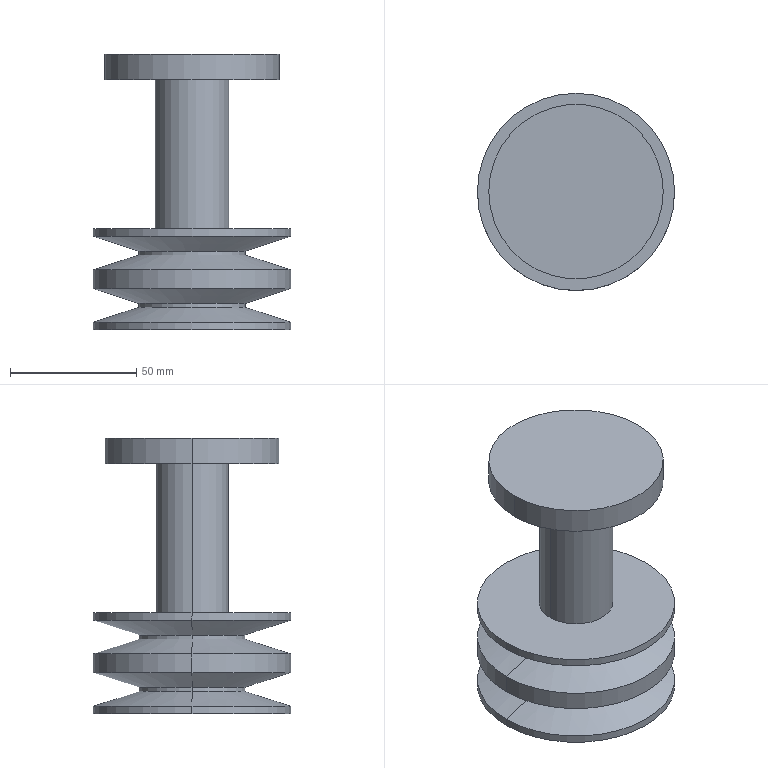Part | SolidWorks | features ICE 6, BaseBody 1 | 1 solid | 38 faces | box 78 x 78 x 109 mm | volume 212709 mm3 | cylinder 18 | cone 11 | plane 9 | commonest cylinder face diameters 78 x6 42 x4 28 x3 29 x2 69 x2 6 x1
STEP:
#1=CARTESIAN_POINT('',(-34.5,0.,109.));
#2=VERTEX_POINT('',#1);
#3=CARTESIAN_POINT('',(34.5,0.,109.));
#4=VERTEX_POINT('',#3);
#5=CARTESIAN_POINT('',(0.,0.,109.));
#6=DIRECTION('',(0.,0.,-1.));
#7=DIRECTION('',(1.,0.,0.));
#8=AXIS2_PLACEMENT_3D('',#5,#6,#7);
#9=CIRCLE('',#8,34.5);
#10=EDGE_CURVE('',#2,#4,#9,.T.);
#11=ORIENTED_EDGE('',*,*,#10,.T.);
#12=CARTESIAN_POINT('',(34.5,0.,99.));
#13=VERTEX_POINT('',#12);
#14=CARTESIAN_POINT('',(34.5,0.,109.));
#15=DIRECTION('',(0.,0.,-1.));
#16=VECTOR('',#15,1000.);
#17=LINE('',#14,#16);
#18=EDGE_CURVE('',#4,#13,#17,.T.);
#19=ORIENTED_EDGE('',*,*,#18,.T.);
#20=CARTESIAN_POINT('',(-34.5,0.,99.));
#21=VERTEX_POINT('',#20);
#22=CARTESIAN_POINT('',(0.,0.,99.));
#23=DIRECTION('',(0.,0.,-1.));
#24=DIRECTION('',(1.,0.,0.));
#25=AXIS2_PLACEMENT_3D('',#22,#23,#24);
#26=CIRCLE('',#25,34.5);
#27=EDGE_CURVE('',#21,#13,#26,.T.);
#28=ORIENTED_EDGE('',*,*,#27,.F.);
#29=CARTESIAN_POINT('',(-34.5,0.,109.));
#30=DIRECTION('',(0.,0.,-1.));
#31=VECTOR('',#30,1000.);
#32=LINE('',#29,#31);
#33=EDGE_CURVE('',#2,#21,#32,.T.);
#34=ORIENTED_EDGE('',*,*,#33,.F.);
#35=EDGE_LOOP('',(#11,#19,#28,#34));
#36=FACE_OUTER_BOUND('',#35,.T.);
#37=CARTESIAN_POINT('',(0.,0.,109.));
#38=DIRECTION('',(0.,0.,-1.));
#39=DIRECTION('',(-1.,0.,0.));
#40=AXIS2_PLACEMENT_3D('',#37,#38,#39);
#41=CYLINDRICAL_SURFACE('',#40,34.5);
#42=ADVANCED_FACE('',(#36),#41,.T.);
#43=CARTESIAN_POINT('',(14.5,0.,99.));
#44=VERTEX_POINT('',#43);
#45=CARTESIAN_POINT('',(-14.5,0.,99.));
#46=VERTEX_POINT('',#45);
#47=CARTESIAN_POINT('',(0.,0.,99.));
#48=DIRECTION('',(0.,0.,1.));
#49=DIRECTION('',(1.,0.,0.));
#50=AXIS2_PLACEMENT_3D('',#47,#48,#49);
#51=CIRCLE('',#50,14.5);
#52=EDGE_CURVE('',#44,#46,#51,.T.);
#53=ORIENTED_EDGE('',*,*,#52,.F.);
#54=CARTESIAN_POINT('',(14.5,0.,40.));
#55=VERTEX_POINT('',#54);
#56=CARTESIAN_POINT('',(14.5,0.,99.));
#57=DIRECTION('',(0.,0.,-1.));
#58=VECTOR('',#57,1000.);
#59=LINE('',#56,#58);
#60=EDGE_CURVE('',#44,#55,#59,.T.);
#61=ORIENTED_EDGE('',*,*,#60,.T.);
#62=CARTESIAN_POINT('',(-14.5,0.,40.));
#63=VERTEX_POINT('',#62);
#64=CARTESIAN_POINT('',(0.,0.,40.));
#65=DIRECTION('',(0.,0.,1.));
#66=DIRECTION('',(1.,0.,0.));
#67=AXIS2_PLACEMENT_3D('',#64,#65,#66);
#68=CIRCLE('',#67,14.5);
#69=EDGE_CURVE('',#55,#63,#68,.T.);
#70=ORIENTED_EDGE('',*,*,#69,.T.);
#71=CARTESIAN_POINT('',(-14.5,0.,99.));
#72=DIRECTION('',(0.,0.,-1.));
#73=VECTOR('',#72,1000.);
#74=LINE('',#71,#73);
#75=EDGE_CURVE('',#46,#63,#74,.T.);
#76=ORIENTED_EDGE('',*,*,#75,.F.);
#77=EDGE_LOOP('',(#53,#61,#70,#76));
#78=FACE_OUTER_BOUND('',#77,.T.);
#79=CARTESIAN_POINT('',(0.,0.,99.));
#80=DIRECTION('',(0.,0.,-1.));
#81=DIRECTION('',(-1.,0.,0.));
#82=AXIS2_PLACEMENT_3D('',#79,#80,#81);
#83=CYLINDRICAL_SURFACE('',#82,14.5);
#84=ADVANCED_FACE('',(#78),#83,.T.);
#85=CARTESIAN_POINT('',(39.,0.,40.));
#86=VERTEX_POINT('',#85);
#87=CARTESIAN_POINT('',(-39.,0.,40.));
#88=VERTEX_POINT('',#87);
#89=CARTESIAN_POINT('',(0.,0.,40.));
#90=DIRECTION('',(0.,0.,1.));
#91=DIRECTION('',(1.,0.,0.));
#92=AXIS2_PLACEMENT_3D('',#89,#90,#91);
#93=CIRCLE('',#92,39.);
#94=EDGE_CURVE('',#86,#88,#93,.T.);
#95=ORIENTED_EDGE('',*,*,#94,.F.);
#96=CARTESIAN_POINT('',(39.,0.,37.));
#97=VERTEX_POINT('',#96);
#98=CARTESIAN_POINT('',(39.,0.,40.));
#99=DIRECTION('',(0.,0.,-1.));
#100=VECTOR('',#99,1000.);
#101=LINE('',#98,#100);
#102=EDGE_CURVE('',#86,#97,#101,.T.);
#103=ORIENTED_EDGE('',*,*,#102,.T.);
#104=CARTESIAN_POINT('',(-39.,0.,37.));
#105=VERTEX_POINT('',#104);
#106=CARTESIAN_POINT('',(0.,0.,37.));
#107=DIRECTION('',(0.,0.,1.));
#108=DIRECTION('',(1.,0.,0.));
#109=AXIS2_PLACEMENT_3D('',#106,#107,#108);
#110=CIRCLE('',#109,39.);
#111=EDGE_CURVE('',#97,#105,#110,.T.);
#112=ORIENTED_EDGE('',*,*,#111,.T.);
#113=CARTESIAN_POINT('',(-39.,0.,40.));
#114=DIRECTION('',(0.,0.,-1.));
#115=VECTOR('',#114,1000.);
#116=LINE('',#113,#115);
#117=EDGE_CURVE('',#88,#105,#116,.T.);
#118=ORIENTED_EDGE('',*,*,#117,.F.);
#119=EDGE_LOOP('',(#95,#103,#112,#118));
#120=FACE_OUTER_BOUND('',#119,.T.);
#121=CARTESIAN_POINT('',(0.,0.,40.));
#122=DIRECTION('',(0.,0.,-1.));
#123=DIRECTION('',(-1.,0.,0.));
#124=AXIS2_PLACEMENT_3D('',#121,#122,#123);
#125=CYLINDRICAL_SURFACE('',#124,39.);
#126=ADVANCED_FACE('',(#120),#125,.T.);
#127=CARTESIAN_POINT('',(-12.,0.,0.));
#128=VERTEX_POINT('',#127);
#129=CARTESIAN_POINT('',(-3.,11.619,0.));
#130=VERTEX_POINT('',#129);
#131=CARTESIAN_POINT('',(0.,0.,0.));
#132=DIRECTION('',(0.,0.,-1.));
#133=DIRECTION('',(1.,0.,0.));
#134=AXIS2_PLACEMENT_3D('',#131,#132,#133);
#135=CIRCLE('',#134,12.);
#136=EDGE_CURVE('',#128,#130,#135,.T.);
#137=ORIENTED_EDGE('',*,*,#136,.F.);
#138=CARTESIAN_POINT('',(-14.,0.,2.));
#139=VERTEX_POINT('',#138);
#140=CARTESIAN_POINT('',(-12.,0.,0.));
#141=DIRECTION('',(-0.7071,0.,0.7071));
#142=VECTOR('',#141,1000.);
#143=LINE('',#140,#142);
#144=EDGE_CURVE('',#128,#139,#143,.T.);
#145=ORIENTED_EDGE('',*,*,#144,.T.);
#146=CARTESIAN_POINT('',(-3.,13.675,2.));
#147=VERTEX_POINT('',#146);
#148=CARTESIAN_POINT('',(0.,0.,2.));
#149=DIRECTION('',(0.,0.,-1.));
#150=DIRECTION('',(-1.,0.,0.));
#151=AXIS2_PLACEMENT_3D('',#148,#149,#150);
#152=CIRCLE('',#151,14.);
#153=EDGE_CURVE('',#139,#147,#152,.T.);
#154=ORIENTED_EDGE('',*,*,#153,.T.);
#155=CARTESIAN_POINT('',(-3.,13.675,2.));
#156=CARTESIAN_POINT('',(-3.,12.991,1.332));
#157=CARTESIAN_POINT('',(-3.,12.306,0.665));
#158=CARTESIAN_POINT('',(-3.,11.619,0.));
#159=B_SPLINE_CURVE_WITH_KNOTS('',3,(#155,#156,#157,#158),.UNSPECIFIED.,.F.,.F.,(4,4),(0.,0.002868),.UNSPECIFIED.);
#160=EDGE_CURVE('',#147,#130,#159,.T.);
#161=ORIENTED_EDGE('',*,*,#160,.T.);
#162=EDGE_LOOP('',(#137,#145,#154,#161));
#163=FACE_OUTER_BOUND('',#162,.T.);
#164=CARTESIAN_POINT('',(0.,0.,0.));
#165=DIRECTION('',(0.,0.,1.));
#166=DIRECTION('',(1.,0.,0.));
#167=AXIS2_PLACEMENT_3D('',#164,#165,#166);
#168=CONICAL_SURFACE('',#167,12.,0.7854);
#169=ADVANCED_FACE('',(#163),#168,.T.);
#170=ORIENTED_EDGE('',*,*,#144,.F.);
#171=CARTESIAN_POINT('',(12.,0.,0.));
#172=VERTEX_POINT('',#171);
#173=CARTESIAN_POINT('',(0.,0.,0.));
#174=DIRECTION('',(0.,0.,-1.));
#175=DIRECTION('',(1.,0.,0.));
#176=AXIS2_PLACEMENT_3D('',#173,#174,#175);
#177=CIRCLE('',#176,12.);
#178=EDGE_CURVE('',#172,#128,#177,.T.);
#179=ORIENTED_EDGE('',*,*,#178,.F.);
#180=CARTESIAN_POINT('',(14.,0.,2.));
#181=VERTEX_POINT('',#180);
#182=CARTESIAN_POINT('',(12.,0.,0.));
#183=DIRECTION('',(0.7071,0.,0.7071));
#184=VECTOR('',#183,1000.);
#185=LINE('',#182,#184);
#186=EDGE_CURVE('',#172,#181,#185,.T.);
#187=ORIENTED_EDGE('',*,*,#186,.T.);
#188=CARTESIAN_POINT('',(0.,0.,2.));
#189=DIRECTION('',(0.,0.,-1.));
#190=DIRECTION('',(-1.,0.,0.));
#191=AXIS2_PLACEMENT_3D('',#188,#189,#190);
#192=CIRCLE('',#191,14.);
#193=EDGE_CURVE('',#181,#139,#192,.T.);
#194=ORIENTED_EDGE('',*,*,#193,.T.);
#195=EDGE_LOOP('',(#170,#179,#187,#194));
#196=FACE_OUTER_BOUND('',#195,.T.);
#197=CARTESIAN_POINT('',(0.,0.,0.));
#198=DIRECTION('',(0.,0.,1.));
#199=DIRECTION('',(1.,0.,0.));
#200=AXIS2_PLACEMENT_3D('',#197,#198,#199);
#201=CONICAL_SURFACE('',#200,12.,0.7854);
#202=ADVANCED_FACE('',(#196),#201,.T.);
#203=CARTESIAN_POINT('',(14.,0.,0.));
#204=VERTEX_POINT('',#203);
#205=CARTESIAN_POINT('',(-14.,0.,0.));
#206=VERTEX_POINT('',#205);
#207=CARTESIAN_POINT('',(0.,0.,0.));
#208=DIRECTION('',(0.,0.,-1.));
#209=DIRECTION('',(1.,0.,0.));
#210=AXIS2_PLACEMENT_3D('',#207,#208,#209);
#211=CIRCLE('',#210,14.);
#212=EDGE_CURVE('',#204,#206,#211,.T.);
#213=ORIENTED_EDGE('',*,*,#212,.T.);
#214=CARTESIAN_POINT('',(-14.,0.,0.));
#215=DIRECTION('',(0.,0.,1.));
#216=VECTOR('',#215,1000.);
#217=LINE('',#214,#216);
#218=EDGE_CURVE('',#206,#139,#217,.T.);
#219=ORIENTED_EDGE('',*,*,#218,.T.);
#220=ORIENTED_EDGE('',*,*,#193,.F.);
#221=CARTESIAN_POINT('',(14.,0.,0.));
#222=DIRECTION('',(0.,0.,1.));
#223=VECTOR('',#222,1000.);
#224=LINE('',#221,#223);
#225=EDGE_CURVE('',#204,#181,#224,.T.);
#226=ORIENTED_EDGE('',*,*,#225,.F.);
#227=EDGE_LOOP('',(#213,#219,#220,#226));
#228=FACE_OUTER_BOUND('',#227,.T.);
#229=CARTESIAN_POINT('',(0.,0.,0.));
#230=DIRECTION('',(0.,0.,1.));
#231=DIRECTION('',(1.,0.,0.));
#232=AXIS2_PLACEMENT_3D('',#229,#230,#231);
#233=CYLINDRICAL_SURFACE('',#232,14.);
#234=ADVANCED_FACE('',(#228),#233,.F.);
#235=CARTESIAN_POINT('',(3.,13.675,0.));
#236=VERTEX_POINT('',#235);
#237=CARTESIAN_POINT('',(0.,0.,0.));
#238=DIRECTION('',(0.,0.,-1.));
#239=DIRECTION('',(1.,0.,0.));
#240=AXIS2_PLACEMENT_3D('',#237,#238,#239);
#241=CIRCLE('',#240,14.);
#242=EDGE_CURVE('',#236,#204,#241,.T.);
#243=ORIENTED_EDGE('',*,*,#242,.T.);
#244=ORIENTED_EDGE('',*,*,#225,.T.);
#245=CARTESIAN_POINT('',(3.,13.675,2.));
#246=VERTEX_POINT('',#245);
#247=CARTESIAN_POINT('',(0.,0.,2.));
#248=DIRECTION('',(0.,0.,-1.));
#249=DIRECTION('',(-1.,0.,0.));
#250=AXIS2_PLACEMENT_3D('',#247,#248,#249);
#251=CIRCLE('',#250,14.);
#252=EDGE_CURVE('',#246,#181,#251,.T.);
#253=ORIENTED_EDGE('',*,*,#252,.F.);
#254=CARTESIAN_POINT('',(3.,13.675,1.));
#255=DIRECTION('',(0.,0.,1.));
#256=VECTOR('',#255,1000.);
#257=LINE('',#254,#256);
#258=EDGE_CURVE('',#236,#246,#257,.T.);
#259=ORIENTED_EDGE('',*,*,#258,.F.);
#260=EDGE_LOOP('',(#243,#244,#253,#259));
#261=FACE_OUTER_BOUND('',#260,.T.);
#262=CARTESIAN_POINT('',(0.,0.,0.));
#263=DIRECTION('',(0.,0.,1.));
#264=DIRECTION('',(1.,0.,0.));
#265=AXIS2_PLACEMENT_3D('',#262,#263,#264);
#266=CYLINDRICAL_SURFACE('',#265,14.);
#267=ADVANCED_FACE('',(#261),#266,.F.);
#268=CARTESIAN_POINT('',(-21.,0.,31.151));
#269=VERTEX_POINT('',#268);
#270=CARTESIAN_POINT('',(21.,0.,31.151));
#271=VERTEX_POINT('',#270);
#272=CARTESIAN_POINT('',(0.,0.,31.151));
#273=DIRECTION('',(0.,0.,-1.));
#274=DIRECTION('',(-1.,0.,0.));
#275=AXIS2_PLACEMENT_3D('',#272,#273,#274);
#276=CIRCLE('',#275,21.);
#277=EDGE_CURVE('',#269,#271,#276,.T.);
#278=ORIENTED_EDGE('',*,*,#277,.F.);
#279=CARTESIAN_POINT('',(-21.,0.,31.151));
#280=DIRECTION('',(-0.9511,0.,0.309));
#281=VECTOR('',#280,1000.);
#282=LINE('',#279,#281);
#283=EDGE_CURVE('',#269,#105,#282,.T.);
#284=ORIENTED_EDGE('',*,*,#283,.T.);
#285=ORIENTED_EDGE('',*,*,#111,.F.);
#286=CARTESIAN_POINT('',(21.,0.,31.151));
#287=DIRECTION('',(0.9511,0.,0.309));
#288=VECTOR('',#287,1000.);
#289=LINE('',#286,#288);
#290=EDGE_CURVE('',#271,#97,#289,.T.);
#291=ORIENTED_EDGE('',*,*,#290,.F.);
#292=EDGE_LOOP('',(#278,#284,#285,#291));
#293=FACE_OUTER_BOUND('',#292,.T.);
#294=CARTESIAN_POINT('',(0.,0.,31.151));
#295=DIRECTION('',(0.,0.,1.));
#296=DIRECTION('',(1.,0.,0.));
#297=AXIS2_PLACEMENT_3D('',#294,#295,#296);
#298=CONICAL_SURFACE('',#297,21.,1.257);
#299=ADVANCED_FACE('',(#293),#298,.T.);
#300=CARTESIAN_POINT('',(-21.,0.,29.549));
#301=VERTEX_POINT('',#300);
#302=CARTESIAN_POINT('',(21.,0.,29.549));
#303=VERTEX_POINT('',#302);
#304=CARTESIAN_POINT('',(0.,0.,29.549));
#305=DIRECTION('',(0.,0.,-1.));
#306=DIRECTION('',(-1.,0.,0.));
#307=AXIS2_PLACEMENT_3D('',#304,#305,#306);
#308=CIRCLE('',#307,21.);
#309=EDGE_CURVE('',#301,#303,#308,.T.);
#310=ORIENTED_EDGE('',*,*,#309,.F.);
#311=CARTESIAN_POINT('',(-21.,0.,29.549));
#312=DIRECTION('',(0.,0.,1.));
#313=VECTOR('',#312,1000.);
#314=LINE('',#311,#313);
#315=EDGE_CURVE('',#301,#269,#314,.T.);
#316=ORIENTED_EDGE('',*,*,#315,.T.);
#317=ORIENTED_EDGE('',*,*,#277,.T.);
#318=CARTESIAN_POINT('',(21.,0.,29.549));
#319=DIRECTION('',(0.,0.,1.));
#320=VECTOR('',#319,1000.);
#321=LINE('',#318,#320);
#322=EDGE_CURVE('',#303,#271,#321,.T.);
#323=ORIENTED_EDGE('',*,*,#322,.F.);
#324=EDGE_LOOP('',(#310,#316,#317,#323));
#325=FACE_OUTER_BOUND('',#324,.T.);
#326=CARTESIAN_POINT('',(0.,0.,29.549));
#327=DIRECTION('',(0.,0.,1.));
#328=DIRECTION('',(1.,0.,0.));
#329=AXIS2_PLACEMENT_3D('',#326,#327,#328);
#330=CYLINDRICAL_SURFACE('',#329,21.);
#331=ADVANCED_FACE('',(#325),#330,.T.);
#332=ORIENTED_EDGE('',*,*,#309,.T.);
#333=CARTESIAN_POINT('',(39.,0.,23.7));
#334=VERTEX_POINT('',#333);
#335=CARTESIAN_POINT('',(39.,0.,23.7));
#336=DIRECTION('',(0.9511,0.,-0.309));
#337=VECTOR('',#336,1000.);
#338=LINE('',#335,#337);
#339=EDGE_CURVE('',#303,#334,#338,.T.);
#340=ORIENTED_EDGE('',*,*,#339,.T.);
#341=CARTESIAN_POINT('',(-39.,0.,23.7));
#342=VERTEX_POINT('',#341);
#343=CARTESIAN_POINT('',(0.,0.,23.7));
#344=DIRECTION('',(0.,0.,-1.));
#345=DIRECTION('',(-1.,0.,0.));
#346=AXIS2_PLACEMENT_3D('',#343,#344,#345);
#347=CIRCLE('',#346,39.);
#348=EDGE_CURVE('',#342,#334,#347,.T.);
#349=ORIENTED_EDGE('',*,*,#348,.F.);
#350=CARTESIAN_POINT('',(-39.,0.,23.7));
#351=DIRECTION('',(-0.9511,0.,-0.309));
#352=VECTOR('',#351,1000.);
#353=LINE('',#350,#352);
#354=EDGE_CURVE('',#301,#342,#353,.T.);
#355=ORIENTED_EDGE('',*,*,#354,.F.);
#356=EDGE_LOOP('',(#332,#340,#349,#355));
#357=FACE_OUTER_BOUND('',#356,.T.);
#358=CARTESIAN_POINT('',(0.,0.,23.7));
#359=DIRECTION('',(0.,0.,-1.));
#360=DIRECTION('',(-1.,0.,0.));
#361=AXIS2_PLACEMENT_3D('',#358,#359,#360);
#362=CONICAL_SURFACE('',#361,39.,1.257);
#363=ADVANCED_FACE('',(#357),#362,.T.);
#364=CARTESIAN_POINT('',(-39.,0.,16.3));
#365=VERTEX_POINT('',#364);
#366=CARTESIAN_POINT('',(39.,0.,16.3));
#367=VERTEX_POINT('',#366);
#368=CARTESIAN_POINT('',(0.,0.,16.3));
#369=DIRECTION('',(0.,0.,-1.));
#370=DIRECTION('',(-1.,0.,0.));
#371=AXIS2_PLACEMENT_3D('',#368,#369,#370);
#372=CIRCLE('',#371,39.);
#373=EDGE_CURVE('',#365,#367,#372,.T.);
#374=ORIENTED_EDGE('',*,*,#373,.F.);
#375=CARTESIAN_POINT('',(-39.,0.,16.3));
#376=DIRECTION('',(0.,0.,1.));
#377=VECTOR('',#376,1000.);
#378=LINE('',#375,#377);
#379=EDGE_CURVE('',#365,#342,#378,.T.);
#380=ORIENTED_EDGE('',*,*,#379,.T.);
#381=ORIENTED_EDGE('',*,*,#348,.T.);
#382=CARTESIAN_POINT('',(39.,0.,16.3));
#383=DIRECTION('',(0.,0.,1.));
#384=VECTOR('',#383,1000.);
#385=LINE('',#382,#384);
#386=EDGE_CURVE('',#367,#334,#385,.T.);
#387=ORIENTED_EDGE('',*,*,#386,.F.);
#388=EDGE_LOOP('',(#374,#380,#381,#387));
#389=FACE_OUTER_BOUND('',#388,.T.);
#390=CARTESIAN_POINT('',(0.,0.,16.3));
#391=DIRECTION('',(0.,0.,1.));
#392=DIRECTION('',(1.,0.,0.));
#393=AXIS2_PLACEMENT_3D('',#390,#391,#392);
#394=CYLINDRICAL_SURFACE('',#393,39.);
#395=ADVANCED_FACE('',(#389),#394,.T.);
#396=CARTESIAN_POINT('',(-21.,0.,10.451));
#397=VERTEX_POINT('',#396);
#398=CARTESIAN_POINT('',(21.,0.,10.451));
#399=VERTEX_POINT('',#398);
#400=CARTESIAN_POINT('',(0.,0.,10.451));
#401=DIRECTION('',(0.,0.,-1.));
#402=DIRECTION('',(-1.,0.,0.));
#403=AXIS2_PLACEMENT_3D('',#400,#401,#402);
#404=CIRCLE('',#403,21.);
#405=EDGE_CURVE('',#397,#399,#404,.T.);
#406=ORIENTED_EDGE('',*,*,#405,.F.);
#407=CARTESIAN_POINT('',(-21.,0.,10.451));
#408=DIRECTION('',(-0.9511,0.,0.309));
#409=VECTOR('',#408,1000.);
#410=LINE('',#407,#409);
#411=EDGE_CURVE('',#397,#365,#410,.T.);
#412=ORIENTED_EDGE('',*,*,#411,.T.);
#413=ORIENTED_EDGE('',*,*,#373,.T.);
#414=CARTESIAN_POINT('',(21.,0.,10.451));
#415=DIRECTION('',(0.9511,0.,0.309));
#416=VECTOR('',#415,1000.);
#417=LINE('',#414,#416);
#418=EDGE_CURVE('',#399,#367,#417,.T.);
#419=ORIENTED_EDGE('',*,*,#418,.F.);
#420=EDGE_LOOP('',(#406,#412,#413,#419));
#421=FACE_OUTER_BOUND('',#420,.T.);
#422=CARTESIAN_POINT('',(0.,0.,10.451));
#423=DIRECTION('',(0.,0.,1.));
#424=DIRECTION('',(1.,0.,0.));
#425=AXIS2_PLACEMENT_3D('',#422,#423,#424);
#426=CONICAL_SURFACE('',#425,21.,1.257);
#427=ADVANCED_FACE('',(#421),#426,.T.);
#428=CARTESIAN_POINT('',(-21.,0.,8.849));
#429=VERTEX_POINT('',#428);
#430=CARTESIAN_POINT('',(21.,0.,8.849));
#431=VERTEX_POINT('',#430);
#432=CARTESIAN_POINT('',(0.,0.,8.849));
#433=DIRECTION('',(0.,0.,-1.));
#434=DIRECTION('',(-1.,0.,0.));
#435=AXIS2_PLACEMENT_3D('',#432,#433,#434);
#436=CIRCLE('',#435,21.);
#437=EDGE_CURVE('',#429,#431,#436,.T.);
#438=ORIENTED_EDGE('',*,*,#437,.F.);
#439=CARTESIAN_POINT('',(-21.,0.,8.849));
#440=DIRECTION('',(0.,0.,1.));
#441=VECTOR('',#440,1000.);
#442=LINE('',#439,#441);
#443=EDGE_CURVE('',#429,#397,#442,.T.);
#444=ORIENTED_EDGE('',*,*,#443,.T.);
#445=ORIENTED_EDGE('',*,*,#405,.T.);
#446=CARTESIAN_POINT('',(21.,0.,8.849));
#447=DIRECTION('',(0.,0.,1.));
#448=VECTOR('',#447,1000.);
#449=LINE('',#446,#448);
#450=EDGE_CURVE('',#431,#399,#449,.T.);
#451=ORIENTED_EDGE('',*,*,#450,.F.);
#452=EDGE_LOOP('',(#438,#444,#445,#451));
#453=FACE_OUTER_BOUND('',#452,.T.);
#454=CARTESIAN_POINT('',(0.,0.,8.849));
#455=DIRECTION('',(0.,0.,1.));
#456=DIRECTION('',(1.,0.,0.));
#457=AXIS2_PLACEMENT_3D('',#454,#455,#456);
#458=CYLINDRICAL_SURFACE('',#457,21.);
#459=ADVANCED_FACE('',(#453),#458,.T.);
#460=ORIENTED_EDGE('',*,*,#437,.T.);
#461=CARTESIAN_POINT('',(39.,0.,3.));
#462=VERTEX_POINT('',#461);
#463=CARTESIAN_POINT('',(39.,0.,3.));
#464=DIRECTION('',(0.9511,0.,-0.309));
#465=VECTOR('',#464,1000.);
#466=LINE('',#463,#465);
#467=EDGE_CURVE('',#431,#462,#466,.T.);
#468=ORIENTED_EDGE('',*,*,#467,.T.);
#469=CARTESIAN_POINT('',(-39.,0.,3.));
#470=VERTEX_POINT('',#469);
#471=CARTESIAN_POINT('',(0.,0.,3.));
#472=DIRECTION('',(0.,0.,-1.));
#473=DIRECTION('',(-1.,0.,0.));
#474=AXIS2_PLACEMENT_3D('',#471,#472,#473);
#475=CIRCLE('',#474,39.);
#476=EDGE_CURVE('',#470,#462,#475,.T.);
#477=ORIENTED_EDGE('',*,*,#476,.F.);
#478=CARTESIAN_POINT('',(-39.,0.,3.));
#479=DIRECTION('',(-0.9511,0.,-0.309));
#480=VECTOR('',#479,1000.);
#481=LINE('',#478,#480);
#482=EDGE_CURVE('',#429,#470,#481,.T.);
#483=ORIENTED_EDGE('',*,*,#482,.F.);
#484=EDGE_LOOP('',(#460,#468,#477,#483));
#485=FACE_OUTER_BOUND('',#484,.T.);
#486=CARTESIAN_POINT('',(0.,0.,3.));
#487=DIRECTION('',(0.,0.,-1.));
#488=DIRECTION('',(-1.,0.,0.));
#489=AXIS2_PLACEMENT_3D('',#486,#487,#488);
#490=CONICAL_SURFACE('',#489,39.,1.257);
#491=ADVANCED_FACE('',(#485),#490,.T.);
#492=CARTESIAN_POINT('',(-39.,0.,0.));
#493=VERTEX_POINT('',#492);
#494=CARTESIAN_POINT('',(39.,0.,0.));
#495=VERTEX_POINT('',#494);
#496=CARTESIAN_POINT('',(0.,0.,0.));
#497=DIRECTION('',(0.,0.,-1.));
#498=DIRECTION('',(1.,0.,0.));
#499=AXIS2_PLACEMENT_3D('',#496,#497,#498);
#500=CIRCLE('',#499,39.);
#501=EDGE_CURVE('',#493,#495,#500,.T.);
#502=ORIENTED_EDGE('',*,*,#501,.F.);
#503=CARTESIAN_POINT('',(-39.,0.,0.));
#504=DIRECTION('',(0.,0.,1.));
#505=VECTOR('',#504,1000.);
#506=LINE('',#503,#505);
#507=EDGE_CURVE('',#493,#470,#506,.T.);
#508=ORIENTED_EDGE('',*,*,#507,.T.);
#509=ORIENTED_EDGE('',*,*,#476,.T.);
#510=CARTESIAN_POINT('',(39.,0.,0.));
#511=DIRECTION('',(0.,0.,1.));
#512=VECTOR('',#511,1000.);
#513=LINE('',#510,#512);
#514=EDGE_CURVE('',#495,#462,#513,.T.);
#515=ORIENTED_EDGE('',*,*,#514,.F.);
#516=EDGE_LOOP('',(#502,#508,#509,#515));
#517=FACE_OUTER_BOUND('',#516,.T.);
#518=CARTESIAN_POINT('',(0.,0.,0.));
#519=DIRECTION('',(0.,0.,1.));
#520=DIRECTION('',(1.,0.,0.));
#521=AXIS2_PLACEMENT_3D('',#518,#519,#520);
#522=CYLINDRICAL_SURFACE('',#521,39.);
#523=ADVANCED_FACE('',(#517),#522,.T.);
#524=CARTESIAN_POINT('',(0.,0.,40.));
#525=DIRECTION('',(0.,0.,1.));
#526=DIRECTION('',(1.,0.,0.));
#527=AXIS2_PLACEMENT_3D('',#524,#525,#526);
#528=CIRCLE('',#527,39.);
#529=EDGE_CURVE('',#88,#86,#528,.T.);
#530=ORIENTED_EDGE('',*,*,#529,.T.);
#531=ORIENTED_EDGE('',*,*,#94,.T.);
#532=EDGE_LOOP('',(#530,#531));
#533=FACE_OUTER_BOUND('',#532,.T.);
#534=CARTESIAN_POINT('',(0.,0.,40.));
#535=DIRECTION('',(0.,0.,1.));
#536=DIRECTION('',(1.,0.,0.));
#537=AXIS2_PLACEMENT_3D('',#534,#535,#536);
#538=CIRCLE('',#537,14.5);
#539=EDGE_CURVE('',#63,#55,#538,.T.);
#540=ORIENTED_EDGE('',*,*,#539,.F.);
#541=ORIENTED_EDGE('',*,*,#69,.F.);
#542=EDGE_LOOP('',(#540,#541));
#543=FACE_BOUND('',#542,.T.);
#544=CARTESIAN_POINT('',(0.,0.,40.));
#545=DIRECTION('',(0.,0.,1.));
#546=DIRECTION('',(1.,0.,0.));
#547=AXIS2_PLACEMENT_3D('',#544,#545,#546);
#548=PLANE('',#547);
#549=ADVANCED_FACE('',(#533,#543),#548,.T.);
#550=ORIENTED_EDGE('',*,*,#242,.F.);
#551=CARTESIAN_POINT('',(3.,17.,0.));
#552=VERTEX_POINT('',#551);
#553=CARTESIAN_POINT('',(3.,17.,0.));
#554=DIRECTION('',(0.,-1.,0.));
#555=VECTOR('',#554,1000.);
#556=LINE('',#553,#555);
#557=EDGE_CURVE('',#552,#236,#556,.T.);
#558=ORIENTED_EDGE('',*,*,#557,.F.);
#559=CARTESIAN_POINT('',(-3.,17.,0.));
#560=VERTEX_POINT('',#559);
#561=CARTESIAN_POINT('',(-3.,17.,0.));
#562=DIRECTION('',(1.,0.,0.));
#563=VECTOR('',#562,1000.);
#564=LINE('',#561,#563);
#565=EDGE_CURVE('',#560,#552,#564,.T.);
#566=ORIENTED_EDGE('',*,*,#565,.F.);
#567=CARTESIAN_POINT('',(-3.,13.675,0.));
#568=VERTEX_POINT('',#567);
#569=CARTESIAN_POINT('',(-3.,17.,0.));
#570=DIRECTION('',(0.,-1.,0.));
#571=VECTOR('',#570,1000.);
#572=LINE('',#569,#571);
#573=EDGE_CURVE('',#560,#568,#572,.T.);
#574=ORIENTED_EDGE('',*,*,#573,.T.);
#575=CARTESIAN_POINT('',(0.,0.,0.));
#576=DIRECTION('',(0.,0.,-1.));
#577=DIRECTION('',(1.,0.,0.));
#578=AXIS2_PLACEMENT_3D('',#575,#576,#577);
#579=CIRCLE('',#578,14.);
#580=EDGE_CURVE('',#206,#568,#579,.T.);
#581=ORIENTED_EDGE('',*,*,#580,.F.);
#582=ORIENTED_EDGE('',*,*,#212,.F.);
#583=EDGE_LOOP('',(#550,#558,#566,#574,#581,#582));
#584=FACE_BOUND('',#583,.T.);
#585=CARTESIAN_POINT('',(0.,0.,0.));
#586=DIRECTION('',(0.,0.,-1.));
#587=DIRECTION('',(1.,0.,0.));
#588=AXIS2_PLACEMENT_3D('',#585,#586,#587);
#589=CIRCLE('',#588,39.);
#590=EDGE_CURVE('',#495,#493,#589,.T.);
#591=ORIENTED_EDGE('',*,*,#590,.T.);
#592=ORIENTED_EDGE('',*,*,#501,.T.);
#593=EDGE_LOOP('',(#591,#592));
#594=FACE_OUTER_BOUND('',#593,.T.);
#595=CARTESIAN_POINT('',(40.56,40.593,0.));
#596=DIRECTION('',(0.,0.,1.));
#597=DIRECTION('',(-1.,0.,0.));
#598=AXIS2_PLACEMENT_3D('',#595,#596,#597);
#599=PLANE('',#598);
#600=ADVANCED_FACE('',(#584,#594),#599,.F.);
#601=ORIENTED_EDGE('',*,*,#283,.F.);
#602=CARTESIAN_POINT('',(0.,0.,31.151));
#603=DIRECTION('',(0.,0.,-1.));
#604=DIRECTION('',(-1.,0.,0.));
#605=AXIS2_PLACEMENT_3D('',#602,#603,#604);
#606=CIRCLE('',#605,21.);
#607=EDGE_CURVE('',#271,#269,#606,.T.);
#608=ORIENTED_EDGE('',*,*,#607,.F.);
#609=ORIENTED_EDGE('',*,*,#290,.T.);
#610=CARTESIAN_POINT('',(0.,0.,37.));
#611=DIRECTION('',(0.,0.,1.));
#612=DIRECTION('',(1.,0.,0.));
#613=AXIS2_PLACEMENT_3D('',#610,#611,#612);
#614=CIRCLE('',#613,39.);
#615=EDGE_CURVE('',#105,#97,#614,.T.);
#616=ORIENTED_EDGE('',*,*,#615,.F.);
#617=EDGE_LOOP('',(#601,#608,#609,#616));
#618=FACE_OUTER_BOUND('',#617,.T.);
#619=CARTESIAN_POINT('',(0.,0.,31.151));
#620=DIRECTION('',(0.,0.,1.));
#621=DIRECTION('',(1.,0.,0.));
#622=AXIS2_PLACEMENT_3D('',#619,#620,#621);
#623=CONICAL_SURFACE('',#622,21.,1.257);
#624=ADVANCED_FACE('',(#618),#623,.T.);
#625=ORIENTED_EDGE('',*,*,#315,.F.);
#626=CARTESIAN_POINT('',(0.,0.,29.549));
#627=DIRECTION('',(0.,0.,-1.));
#628=DIRECTION('',(-1.,0.,0.));
#629=AXIS2_PLACEMENT_3D('',#626,#627,#628);
#630=CIRCLE('',#629,21.);
#631=EDGE_CURVE('',#303,#301,#630,.T.);
#632=ORIENTED_EDGE('',*,*,#631,.F.);
#633=ORIENTED_EDGE('',*,*,#322,.T.);
#634=ORIENTED_EDGE('',*,*,#607,.T.);
#635=EDGE_LOOP('',(#625,#632,#633,#634));
#636=FACE_OUTER_BOUND('',#635,.T.);
#637=CARTESIAN_POINT('',(0.,0.,29.549));
#638=DIRECTION('',(0.,0.,1.));
#639=DIRECTION('',(1.,0.,0.));
#640=AXIS2_PLACEMENT_3D('',#637,#638,#639);
#641=CYLINDRICAL_SURFACE('',#640,21.);
#642=ADVANCED_FACE('',(#636),#641,.T.);
#643=ORIENTED_EDGE('',*,*,#339,.F.);
#644=ORIENTED_EDGE('',*,*,#631,.T.);
#645=ORIENTED_EDGE('',*,*,#354,.T.);
#646=CARTESIAN_POINT('',(0.,0.,23.7));
#647=DIRECTION('',(0.,0.,-1.));
#648=DIRECTION('',(-1.,0.,0.));
#649=AXIS2_PLACEMENT_3D('',#646,#647,#648);
#650=CIRCLE('',#649,39.);
#651=EDGE_CURVE('',#334,#342,#650,.T.);
#652=ORIENTED_EDGE('',*,*,#651,.F.);
#653=EDGE_LOOP('',(#643,#644,#645,#652));
#654=FACE_OUTER_BOUND('',#653,.T.);
#655=CARTESIAN_POINT('',(0.,0.,23.7));
#656=DIRECTION('',(0.,0.,-1.));
#657=DIRECTION('',(-1.,0.,0.));
#658=AXIS2_PLACEMENT_3D('',#655,#656,#657);
#659=CONICAL_SURFACE('',#658,39.,1.257);
#660=ADVANCED_FACE('',(#654),#659,.T.);
#661=ORIENTED_EDGE('',*,*,#379,.F.);
#662=CARTESIAN_POINT('',(0.,0.,16.3));
#663=DIRECTION('',(0.,0.,-1.));
#664=DIRECTION('',(-1.,0.,0.));
#665=AXIS2_PLACEMENT_3D('',#662,#663,#664);
#666=CIRCLE('',#665,39.);
#667=EDGE_CURVE('',#367,#365,#666,.T.);
#668=ORIENTED_EDGE('',*,*,#667,.F.);
#669=ORIENTED_EDGE('',*,*,#386,.T.);
#670=ORIENTED_EDGE('',*,*,#651,.T.);
#671=EDGE_LOOP('',(#661,#668,#669,#670));
#672=FACE_OUTER_BOUND('',#671,.T.);
#673=CARTESIAN_POINT('',(0.,0.,16.3));
#674=DIRECTION('',(0.,0.,1.));
#675=DIRECTION('',(1.,0.,0.));
#676=AXIS2_PLACEMENT_3D('',#673,#674,#675);
#677=CYLINDRICAL_SURFACE('',#676,39.);
#678=ADVANCED_FACE('',(#672),#677,.T.);
#679=ORIENTED_EDGE('',*,*,#411,.F.);
#680=CARTESIAN_POINT('',(0.,0.,10.451));
#681=DIRECTION('',(0.,0.,-1.));
#682=DIRECTION('',(-1.,0.,0.));
#683=AXIS2_PLACEMENT_3D('',#680,#681,#682);
#684=CIRCLE('',#683,21.);
#685=EDGE_CURVE('',#399,#397,#684,.T.);
#686=ORIENTED_EDGE('',*,*,#685,.F.);
#687=ORIENTED_EDGE('',*,*,#418,.T.);
#688=ORIENTED_EDGE('',*,*,#667,.T.);
#689=EDGE_LOOP('',(#679,#686,#687,#688));
#690=FACE_OUTER_BOUND('',#689,.T.);
#691=CARTESIAN_POINT('',(0.,0.,10.451));
#692=DIRECTION('',(0.,0.,1.));
#693=DIRECTION('',(1.,0.,0.));
#694=AXIS2_PLACEMENT_3D('',#691,#692,#693);
#695=CONICAL_SURFACE('',#694,21.,1.257);
#696=ADVANCED_FACE('',(#690),#695,.T.);
#697=ORIENTED_EDGE('',*,*,#443,.F.);
#698=CARTESIAN_POINT('',(0.,0.,8.849));
#699=DIRECTION('',(0.,0.,-1.));
#700=DIRECTION('',(-1.,0.,0.));
#701=AXIS2_PLACEMENT_3D('',#698,#699,#700);
#702=CIRCLE('',#701,21.);
#703=EDGE_CURVE('',#431,#429,#702,.T.);
#704=ORIENTED_EDGE('',*,*,#703,.F.);
#705=ORIENTED_EDGE('',*,*,#450,.T.);
#706=ORIENTED_EDGE('',*,*,#685,.T.);
#707=EDGE_LOOP('',(#697,#704,#705,#706));
#708=FACE_OUTER_BOUND('',#707,.T.);
#709=CARTESIAN_POINT('',(0.,0.,8.849));
#710=DIRECTION('',(0.,0.,1.));
#711=DIRECTION('',(1.,0.,0.));
#712=AXIS2_PLACEMENT_3D('',#709,#710,#711);
#713=CYLINDRICAL_SURFACE('',#712,21.);
#714=ADVANCED_FACE('',(#708),#713,.T.);
#715=ORIENTED_EDGE('',*,*,#467,.F.);
#716=ORIENTED_EDGE('',*,*,#703,.T.);
#717=ORIENTED_EDGE('',*,*,#482,.T.);
#718=CARTESIAN_POINT('',(0.,0.,3.));
#719=DIRECTION('',(0.,0.,-1.));
#720=DIRECTION('',(-1.,0.,0.));
#721=AXIS2_PLACEMENT_3D('',#718,#719,#720);
#722=CIRCLE('',#721,39.);
#723=EDGE_CURVE('',#462,#470,#722,.T.);
#724=ORIENTED_EDGE('',*,*,#723,.F.);
#725=EDGE_LOOP('',(#715,#716,#717,#724));
#726=FACE_OUTER_BOUND('',#725,.T.);
#727=CARTESIAN_POINT('',(0.,0.,3.));
#728=DIRECTION('',(0.,0.,-1.));
#729=DIRECTION('',(-1.,0.,0.));
#730=AXIS2_PLACEMENT_3D('',#727,#728,#729);
#731=CONICAL_SURFACE('',#730,39.,1.257);
#732=ADVANCED_FACE('',(#726),#731,.T.);
#733=ORIENTED_EDGE('',*,*,#507,.F.);
#734=ORIENTED_EDGE('',*,*,#590,.F.);
#735=ORIENTED_EDGE('',*,*,#514,.T.);
#736=ORIENTED_EDGE('',*,*,#723,.T.);
#737=EDGE_LOOP('',(#733,#734,#735,#736));
#738=FACE_OUTER_BOUND('',#737,.T.);
#739=CARTESIAN_POINT('',(0.,0.,0.));
#740=DIRECTION('',(0.,0.,1.));
#741=DIRECTION('',(1.,0.,0.));
#742=AXIS2_PLACEMENT_3D('',#739,#740,#741);
#743=CYLINDRICAL_SURFACE('',#742,39.);
#744=ADVANCED_FACE('',(#738),#743,.T.);
#745=CARTESIAN_POINT('',(3.,11.619,0.));
#746=VERTEX_POINT('',#745);
#747=CARTESIAN_POINT('',(0.,0.,0.));
#748=DIRECTION('',(0.,0.,-1.));
#749=DIRECTION('',(1.,0.,0.));
#750=AXIS2_PLACEMENT_3D('',#747,#748,#749);
#751=CIRCLE('',#750,12.);
#752=EDGE_CURVE('',#746,#172,#751,.T.);
#753=ORIENTED_EDGE('',*,*,#752,.T.);
#754=ORIENTED_EDGE('',*,*,#178,.T.);
#755=ORIENTED_EDGE('',*,*,#136,.T.);
#756=CARTESIAN_POINT('',(-3.,11.,0.));
#757=VERTEX_POINT('',#756);
#758=CARTESIAN_POINT('',(-3.,11.,0.));
#759=DIRECTION('',(0.,1.,0.));
#760=VECTOR('',#759,1000.);
#761=LINE('',#758,#760);
#762=EDGE_CURVE('',#757,#130,#761,.T.);
#763=ORIENTED_EDGE('',*,*,#762,.F.);
#764=CARTESIAN_POINT('',(3.,11.,0.));
#765=VERTEX_POINT('',#764);
#766=CARTESIAN_POINT('',(3.,11.,0.));
#767=DIRECTION('',(-1.,0.,0.));
#768=VECTOR('',#767,1000.);
#769=LINE('',#766,#768);
#770=EDGE_CURVE('',#765,#757,#769,.T.);
#771=ORIENTED_EDGE('',*,*,#770,.F.);
#772=CARTESIAN_POINT('',(3.,11.,0.));
#773=DIRECTION('',(0.,1.,0.));
#774=VECTOR('',#773,1000.);
#775=LINE('',#772,#774);
#776=EDGE_CURVE('',#765,#746,#775,.T.);
#777=ORIENTED_EDGE('',*,*,#776,.T.);
#778=EDGE_LOOP('',(#753,#754,#755,#763,#771,#777));
#779=FACE_OUTER_BOUND('',#778,.T.);
#780=CARTESIAN_POINT('',(40.56,40.593,0.));
#781=DIRECTION('',(0.,0.,1.));
#782=DIRECTION('',(-1.,0.,0.));
#783=AXIS2_PLACEMENT_3D('',#780,#781,#782);
#784=PLANE('',#783);
#785=ADVANCED_FACE('',(#779),#784,.F.);
#786=ORIENTED_EDGE('',*,*,#218,.F.);
#787=ORIENTED_EDGE('',*,*,#580,.T.);
#788=CARTESIAN_POINT('',(-3.,13.675,2.57));
#789=DIRECTION('',(0.,0.,1.));
#790=VECTOR('',#789,1000.);
#791=LINE('',#788,#790);
#792=EDGE_CURVE('',#568,#147,#791,.T.);
#793=ORIENTED_EDGE('',*,*,#792,.T.);
#794=ORIENTED_EDGE('',*,*,#153,.F.);
#795=EDGE_LOOP('',(#786,#787,#793,#794));
#796=FACE_OUTER_BOUND('',#795,.T.);
#797=CARTESIAN_POINT('',(0.,0.,0.));
#798=DIRECTION('',(0.,0.,1.));
#799=DIRECTION('',(1.,0.,0.));
#800=AXIS2_PLACEMENT_3D('',#797,#798,#799);
#801=CYLINDRICAL_SURFACE('',#800,14.);
#802=ADVANCED_FACE('',(#796),#801,.F.);
#803=ORIENTED_EDGE('',*,*,#186,.F.);
#804=ORIENTED_EDGE('',*,*,#752,.F.);
#805=CARTESIAN_POINT('',(3.,11.619,0.));
#806=CARTESIAN_POINT('',(3.,12.306,0.665));
#807=CARTESIAN_POINT('',(3.,12.991,1.332));
#808=CARTESIAN_POINT('',(3.,13.675,2.));
#809=B_SPLINE_CURVE_WITH_KNOTS('',3,(#805,#806,#807,#808),.UNSPECIFIED.,.F.,.F.,(4,4),(0.,0.002868),.UNSPECIFIED.);
#810=EDGE_CURVE('',#746,#246,#809,.T.);
#811=ORIENTED_EDGE('',*,*,#810,.T.);
#812=ORIENTED_EDGE('',*,*,#252,.T.);
#813=EDGE_LOOP('',(#803,#804,#811,#812));
#814=FACE_OUTER_BOUND('',#813,.T.);
#815=CARTESIAN_POINT('',(0.,0.,0.));
#816=DIRECTION('',(0.,0.,1.));
#817=DIRECTION('',(1.,0.,0.));
#818=AXIS2_PLACEMENT_3D('',#815,#816,#817);
#819=CONICAL_SURFACE('',#818,12.,0.7854);
#820=ADVANCED_FACE('',(#814),#819,.T.);
#821=ORIENTED_EDGE('',*,*,#102,.F.);
#822=ORIENTED_EDGE('',*,*,#529,.F.);
#823=ORIENTED_EDGE('',*,*,#117,.T.);
#824=ORIENTED_EDGE('',*,*,#615,.T.);
#825=EDGE_LOOP('',(#821,#822,#823,#824));
#826=FACE_OUTER_BOUND('',#825,.T.);
#827=CARTESIAN_POINT('',(0.,0.,40.));
#828=DIRECTION('',(0.,0.,-1.));
#829=DIRECTION('',(-1.,0.,0.));
#830=AXIS2_PLACEMENT_3D('',#827,#828,#829);
#831=CYLINDRICAL_SURFACE('',#830,39.);
#832=ADVANCED_FACE('',(#826),#831,.T.);
#833=ORIENTED_EDGE('',*,*,#160,.F.);
#834=ORIENTED_EDGE('',*,*,#792,.F.);
#835=ORIENTED_EDGE('',*,*,#573,.F.);
#836=CARTESIAN_POINT('',(-3.,17.,5.14));
#837=VERTEX_POINT('',#836);
#838=CARTESIAN_POINT('',(-3.,17.,5.14));
#839=DIRECTION('',(0.,0.,-1.));
#840=VECTOR('',#839,1000.);
#841=LINE('',#838,#840);
#842=EDGE_CURVE('',#837,#560,#841,.T.);
#843=ORIENTED_EDGE('',*,*,#842,.F.);
#844=CARTESIAN_POINT('',(-3.,11.,5.14));
#845=VERTEX_POINT('',#844);
#846=CARTESIAN_POINT('',(-3.,11.619,5.14));
#847=DIRECTION('',(0.,1.,0.));
#848=VECTOR('',#847,1000.);
#849=LINE('',#846,#848);
#850=EDGE_CURVE('',#845,#837,#849,.T.);
#851=ORIENTED_EDGE('',*,*,#850,.F.);
#852=CARTESIAN_POINT('',(-3.,11.,0.));
#853=DIRECTION('',(0.,0.,1.));
#854=VECTOR('',#853,1000.);
#855=LINE('',#852,#854);
#856=EDGE_CURVE('',#757,#845,#855,.T.);
#857=ORIENTED_EDGE('',*,*,#856,.F.);
#858=ORIENTED_EDGE('',*,*,#762,.T.);
#859=EDGE_LOOP('',(#833,#834,#835,#843,#851,#857,#858));
#860=FACE_OUTER_BOUND('',#859,.T.);
#861=CARTESIAN_POINT('',(-3.,11.619,0.));
#862=DIRECTION('',(-1.,0.,0.));
#863=DIRECTION('',(0.,0.,1.));
#864=AXIS2_PLACEMENT_3D('',#861,#862,#863);
#865=PLANE('',#864);
#866=ADVANCED_FACE('',(#860),#865,.F.);
#867=ORIENTED_EDGE('',*,*,#810,.F.);
#868=ORIENTED_EDGE('',*,*,#776,.F.);
#869=CARTESIAN_POINT('',(3.,11.,5.14));
#870=VERTEX_POINT('',#869);
#871=CARTESIAN_POINT('',(3.,11.,5.14));
#872=DIRECTION('',(0.,0.,-1.));
#873=VECTOR('',#872,1000.);
#874=LINE('',#871,#873);
#875=EDGE_CURVE('',#870,#765,#874,.T.);
#876=ORIENTED_EDGE('',*,*,#875,.F.);
#877=CARTESIAN_POINT('',(3.,17.,5.14));
#878=VERTEX_POINT('',#877);
#879=CARTESIAN_POINT('',(3.,11.619,5.14));
#880=DIRECTION('',(0.,1.,0.));
#881=VECTOR('',#880,1000.);
#882=LINE('',#879,#881);
#883=EDGE_CURVE('',#870,#878,#882,.T.);
#884=ORIENTED_EDGE('',*,*,#883,.T.);
#885=CARTESIAN_POINT('',(3.,17.,0.));
#886=DIRECTION('',(0.,0.,1.));
#887=VECTOR('',#886,1000.);
#888=LINE('',#885,#887);
#889=EDGE_CURVE('',#552,#878,#888,.T.);
#890=ORIENTED_EDGE('',*,*,#889,.F.);
#891=ORIENTED_EDGE('',*,*,#557,.T.);
#892=ORIENTED_EDGE('',*,*,#258,.T.);
#893=EDGE_LOOP('',(#867,#868,#876,#884,#890,#891,#892));
#894=FACE_OUTER_BOUND('',#893,.T.);
#895=CARTESIAN_POINT('',(3.,11.619,5.14));
#896=DIRECTION('',(1.,0.,0.));
#897=DIRECTION('',(0.,0.,-1.));
#898=AXIS2_PLACEMENT_3D('',#895,#896,#897);
#899=PLANE('',#898);
#900=ADVANCED_FACE('',(#894),#899,.F.);
#901=ORIENTED_EDGE('',*,*,#850,.T.);
#902=CARTESIAN_POINT('',(0.,17.,5.14));
#903=DIRECTION('',(0.,1.,0.));
#904=DIRECTION('',(0.,0.,1.));
#905=AXIS2_PLACEMENT_3D('',#902,#903,#904);
#906=CIRCLE('',#905,3.);
#907=EDGE_CURVE('',#878,#837,#906,.T.);
#908=ORIENTED_EDGE('',*,*,#907,.F.);
#909=ORIENTED_EDGE('',*,*,#883,.F.);
#910=CARTESIAN_POINT('',(0.,11.,5.14));
#911=DIRECTION('',(0.,-1.,0.));
#912=DIRECTION('',(0.,0.,-1.));
#913=AXIS2_PLACEMENT_3D('',#910,#911,#912);
#914=CIRCLE('',#913,3.);
#915=EDGE_CURVE('',#845,#870,#914,.T.);
#916=ORIENTED_EDGE('',*,*,#915,.F.);
#917=EDGE_LOOP('',(#901,#908,#909,#916));
#918=FACE_OUTER_BOUND('',#917,.T.);
#919=CARTESIAN_POINT('',(0.,11.619,5.14));
#920=DIRECTION('',(0.,1.,0.));
#921=DIRECTION('',(0.,0.,1.));
#922=AXIS2_PLACEMENT_3D('',#919,#920,#921);
#923=CYLINDRICAL_SURFACE('',#922,3.);
#924=ADVANCED_FACE('',(#918),#923,.T.);
#925=ORIENTED_EDGE('',*,*,#60,.F.);
#926=CARTESIAN_POINT('',(0.,0.,99.));
#927=DIRECTION('',(0.,0.,1.));
#928=DIRECTION('',(1.,0.,0.));
#929=AXIS2_PLACEMENT_3D('',#926,#927,#928);
#930=CIRCLE('',#929,14.5);
#931=EDGE_CURVE('',#46,#44,#930,.T.);
#932=ORIENTED_EDGE('',*,*,#931,.F.);
#933=ORIENTED_EDGE('',*,*,#75,.T.);
#934=ORIENTED_EDGE('',*,*,#539,.T.);
#935=EDGE_LOOP('',(#925,#932,#933,#934));
#936=FACE_OUTER_BOUND('',#935,.T.);
#937=CARTESIAN_POINT('',(0.,0.,99.));
#938=DIRECTION('',(0.,0.,-1.));
#939=DIRECTION('',(-1.,0.,0.));
#940=AXIS2_PLACEMENT_3D('',#937,#938,#939);
#941=CYLINDRICAL_SURFACE('',#940,14.5);
#942=ADVANCED_FACE('',(#936),#941,.T.);
#943=ORIENTED_EDGE('',*,*,#915,.T.);
#944=ORIENTED_EDGE('',*,*,#875,.T.);
#945=ORIENTED_EDGE('',*,*,#770,.T.);
#946=ORIENTED_EDGE('',*,*,#856,.T.);
#947=EDGE_LOOP('',(#943,#944,#945,#946));
#948=FACE_OUTER_BOUND('',#947,.T.);
#949=CARTESIAN_POINT('',(0.,11.,5.14));
#950=DIRECTION('',(0.,-1.,0.));
#951=DIRECTION('',(0.,0.,-1.));
#952=AXIS2_PLACEMENT_3D('',#949,#950,#951);
#953=PLANE('',#952);
#954=ADVANCED_FACE('',(#948),#953,.F.);
#955=ORIENTED_EDGE('',*,*,#907,.T.);
#956=ORIENTED_EDGE('',*,*,#842,.T.);
#957=ORIENTED_EDGE('',*,*,#565,.T.);
#958=ORIENTED_EDGE('',*,*,#889,.T.);
#959=EDGE_LOOP('',(#955,#956,#957,#958));
#960=FACE_OUTER_BOUND('',#959,.T.);
#961=CARTESIAN_POINT('',(0.,17.,5.14));
#962=DIRECTION('',(0.,1.,0.));
#963=DIRECTION('',(0.,0.,1.));
#964=AXIS2_PLACEMENT_3D('',#961,#962,#963);
#965=PLANE('',#964);
#966=ADVANCED_FACE('',(#960),#965,.F.);
#967=ORIENTED_EDGE('',*,*,#27,.T.);
#968=CARTESIAN_POINT('',(0.,0.,99.));
#969=DIRECTION('',(0.,0.,-1.));
#970=DIRECTION('',(1.,0.,0.));
#971=AXIS2_PLACEMENT_3D('',#968,#969,#970);
#972=CIRCLE('',#971,34.5);
#973=EDGE_CURVE('',#13,#21,#972,.T.);
#974=ORIENTED_EDGE('',*,*,#973,.T.);
#975=EDGE_LOOP('',(#967,#974));
#976=FACE_OUTER_BOUND('',#975,.T.);
#977=ORIENTED_EDGE('',*,*,#931,.T.);
#978=ORIENTED_EDGE('',*,*,#52,.T.);
#979=EDGE_LOOP('',(#977,#978));
#980=FACE_BOUND('',#979,.T.);
#981=CARTESIAN_POINT('',(0.,0.,99.));
#982=DIRECTION('',(0.,0.,1.));
#983=DIRECTION('',(1.,0.,0.));
#984=AXIS2_PLACEMENT_3D('',#981,#982,#983);
#985=PLANE('',#984);
#986=ADVANCED_FACE('',(#976,#980),#985,.F.);
#987=ORIENTED_EDGE('',*,*,#18,.F.);
#988=CARTESIAN_POINT('',(0.,0.,109.));
#989=DIRECTION('',(0.,0.,-1.));
#990=DIRECTION('',(1.,0.,0.));
#991=AXIS2_PLACEMENT_3D('',#988,#989,#990);
#992=CIRCLE('',#991,34.5);
#993=EDGE_CURVE('',#4,#2,#992,.T.);
#994=ORIENTED_EDGE('',*,*,#993,.T.);
#995=ORIENTED_EDGE('',*,*,#33,.T.);
#996=ORIENTED_EDGE('',*,*,#973,.F.);
#997=EDGE_LOOP('',(#987,#994,#995,#996));
#998=FACE_OUTER_BOUND('',#997,.T.);
#999=CARTESIAN_POINT('',(0.,0.,109.));
#1000=DIRECTION('',(0.,0.,-1.));
#1001=DIRECTION('',(-1.,0.,0.));
#1002=AXIS2_PLACEMENT_3D('',#999,#1000,#1001);
#1003=CYLINDRICAL_SURFACE('',#1002,34.5);
#1004=ADVANCED_FACE('',(#998),#1003,.T.);
#1005=ORIENTED_EDGE('',*,*,#10,.F.);
#1006=ORIENTED_EDGE('',*,*,#993,.F.);
#1007=EDGE_LOOP('',(#1005,#1006));
#1008=FACE_OUTER_BOUND('',#1007,.T.);
#1009=CARTESIAN_POINT('',(0.,0.,109.));
#1010=DIRECTION('',(0.,0.,1.));
#1011=DIRECTION('',(1.,0.,0.));
#1012=AXIS2_PLACEMENT_3D('',#1009,#1010,#1011);
#1013=PLANE('',#1012);
#1014=ADVANCED_FACE('',(#1008),#1013,.T.);
#1015=CLOSED_SHELL('',(#42,#84,#126,#169,#202,#234,#267,#299,#331,#363,#395,#427,#459,#491,#523,#549,#600,#624,#642,#660,#678,#696,#714,#732,#744,#785,#802,#820,#832,#866,#900,#924,#942,#954,#966,#986,#1004,#1014));
#1016=MANIFOLD_SOLID_BREP('',#1015);
#1017=CARTESIAN_POINT('',(0.,0.,0.));
#1018=DIRECTION('',(0.,0.,1.));
#1019=DIRECTION('',(1.,0.,0.));
#1020=AXIS2_PLACEMENT_3D('',#1017,#1018,#1019);
#1021=(LENGTH_UNIT()NAMED_UNIT(*)SI_UNIT(.MILLI.,.METRE.));
#1022=UNCERTAINTY_MEASURE_WITH_UNIT(LENGTH_MEASURE(0.00001),#1021,'','');
#1023=(NAMED_UNIT(*)PLANE_ANGLE_UNIT()SI_UNIT($,.RADIAN.));
#1024=(NAMED_UNIT(*)SI_UNIT($,.STERADIAN.)SOLID_ANGLE_UNIT());
#1025=(GEOMETRIC_REPRESENTATION_CONTEXT(3)GLOBAL_UNCERTAINTY_ASSIGNED_CONTEXT((#1022))GLOBAL_UNIT_ASSIGNED_CONTEXT((#1021,#1023,#1024))REPRESENTATION_CONTEXT('',''));
#1026=ADVANCED_BREP_SHAPE_REPRESENTATION('',(#1016,#1020),#1025);